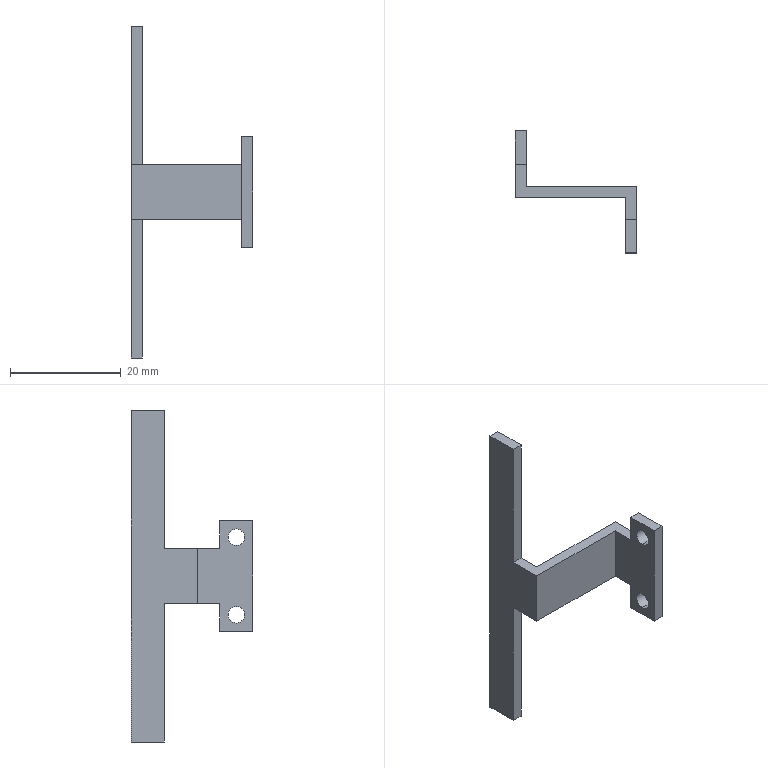Part | SolidWorks | features ICE 2, Extrusion 1 | 1 solid | 22 faces | box 22 x 22 x 60 mm | volume 1532 mm3 | plane 18 | cylinder 4 | commonest cylinder face diameters 3 x4
STEP:
#1=CARTESIAN_POINT('',(3.784,-3.326,8.5));
#2=VERTEX_POINT('',#1);
#3=CARTESIAN_POINT('',(3.784,-3.326,5.5));
#4=VERTEX_POINT('',#3);
#5=CARTESIAN_POINT('',(3.784,-3.326,7.));
#6=DIRECTION('',(1.,0.,0.));
#7=DIRECTION('',(0.,0.,-1.));
#8=AXIS2_PLACEMENT_3D('',#5,#6,#7);
#9=CIRCLE('',#8,1.5);
#10=EDGE_CURVE('',#2,#4,#9,.T.);
#11=ORIENTED_EDGE('',*,*,#10,.F.);
#12=CARTESIAN_POINT('',(5.784,-3.326,8.5));
#13=VERTEX_POINT('',#12);
#14=CARTESIAN_POINT('',(3.784,-3.326,8.5));
#15=DIRECTION('',(1.,0.,0.));
#16=VECTOR('',#15,1000.);
#17=LINE('',#14,#16);
#18=EDGE_CURVE('',#2,#13,#17,.T.);
#19=ORIENTED_EDGE('',*,*,#18,.T.);
#20=CARTESIAN_POINT('',(5.784,-3.326,5.5));
#21=VERTEX_POINT('',#20);
#22=CARTESIAN_POINT('',(5.784,-3.326,7.));
#23=DIRECTION('',(1.,0.,0.));
#24=DIRECTION('',(0.,0.,-1.));
#25=AXIS2_PLACEMENT_3D('',#22,#23,#24);
#26=CIRCLE('',#25,1.5);
#27=EDGE_CURVE('',#13,#21,#26,.T.);
#28=ORIENTED_EDGE('',*,*,#27,.T.);
#29=CARTESIAN_POINT('',(3.784,-3.326,5.5));
#30=DIRECTION('',(1.,0.,0.));
#31=VECTOR('',#30,1000.);
#32=LINE('',#29,#31);
#33=EDGE_CURVE('',#4,#21,#32,.T.);
#34=ORIENTED_EDGE('',*,*,#33,.F.);
#35=EDGE_LOOP('',(#11,#19,#28,#34));
#36=FACE_OUTER_BOUND('',#35,.T.);
#37=CARTESIAN_POINT('',(3.784,-3.326,7.));
#38=DIRECTION('',(1.,0.,0.));
#39=DIRECTION('',(0.,0.,-1.));
#40=AXIS2_PLACEMENT_3D('',#37,#38,#39);
#41=CYLINDRICAL_SURFACE('',#40,1.5);
#42=ADVANCED_FACE('',(#36),#41,.F.);
#43=CARTESIAN_POINT('',(3.784,-3.326,-5.5));
#44=VERTEX_POINT('',#43);
#45=CARTESIAN_POINT('',(3.784,-3.326,-8.5));
#46=VERTEX_POINT('',#45);
#47=CARTESIAN_POINT('',(3.784,-3.326,-7.));
#48=DIRECTION('',(1.,0.,0.));
#49=DIRECTION('',(0.,0.,-1.));
#50=AXIS2_PLACEMENT_3D('',#47,#48,#49);
#51=CIRCLE('',#50,1.5);
#52=EDGE_CURVE('',#44,#46,#51,.T.);
#53=ORIENTED_EDGE('',*,*,#52,.F.);
#54=CARTESIAN_POINT('',(5.784,-3.326,-5.5));
#55=VERTEX_POINT('',#54);
#56=CARTESIAN_POINT('',(3.784,-3.326,-5.5));
#57=DIRECTION('',(1.,0.,0.));
#58=VECTOR('',#57,1000.);
#59=LINE('',#56,#58);
#60=EDGE_CURVE('',#44,#55,#59,.T.);
#61=ORIENTED_EDGE('',*,*,#60,.T.);
#62=CARTESIAN_POINT('',(5.784,-3.326,-8.5));
#63=VERTEX_POINT('',#62);
#64=CARTESIAN_POINT('',(5.784,-3.326,-7.));
#65=DIRECTION('',(1.,0.,0.));
#66=DIRECTION('',(0.,0.,-1.));
#67=AXIS2_PLACEMENT_3D('',#64,#65,#66);
#68=CIRCLE('',#67,1.5);
#69=EDGE_CURVE('',#55,#63,#68,.T.);
#70=ORIENTED_EDGE('',*,*,#69,.T.);
#71=CARTESIAN_POINT('',(3.784,-3.326,-8.5));
#72=DIRECTION('',(1.,0.,0.));
#73=VECTOR('',#72,1000.);
#74=LINE('',#71,#73);
#75=EDGE_CURVE('',#46,#63,#74,.T.);
#76=ORIENTED_EDGE('',*,*,#75,.F.);
#77=EDGE_LOOP('',(#53,#61,#70,#76));
#78=FACE_OUTER_BOUND('',#77,.T.);
#79=CARTESIAN_POINT('',(3.784,-3.326,-7.));
#80=DIRECTION('',(1.,0.,0.));
#81=DIRECTION('',(0.,0.,-1.));
#82=AXIS2_PLACEMENT_3D('',#79,#80,#81);
#83=CYLINDRICAL_SURFACE('',#82,1.5);
#84=ADVANCED_FACE('',(#78),#83,.F.);
#85=CARTESIAN_POINT('',(5.784,-0.3262,5.));
#86=VERTEX_POINT('',#85);
#87=CARTESIAN_POINT('',(5.784,5.674,5.));
#88=VERTEX_POINT('',#87);
#89=CARTESIAN_POINT('',(5.784,5.674,5.));
#90=DIRECTION('',(0.,1.,0.));
#91=VECTOR('',#90,1000.);
#92=LINE('',#89,#91);
#93=EDGE_CURVE('',#86,#88,#92,.T.);
#94=ORIENTED_EDGE('',*,*,#93,.F.);
#95=CARTESIAN_POINT('',(5.784,-0.3262,10.));
#96=VERTEX_POINT('',#95);
#97=CARTESIAN_POINT('',(5.784,-0.3262,-10.));
#98=DIRECTION('',(0.,0.,1.));
#99=VECTOR('',#98,1000.);
#100=LINE('',#97,#99);
#101=EDGE_CURVE('',#86,#96,#100,.T.);
#102=ORIENTED_EDGE('',*,*,#101,.T.);
#103=CARTESIAN_POINT('',(5.784,-6.326,10.));
#104=VERTEX_POINT('',#103);
#105=CARTESIAN_POINT('',(5.784,-0.3262,10.));
#106=DIRECTION('',(0.,-1.,0.));
#107=VECTOR('',#106,1000.);
#108=LINE('',#105,#107);
#109=EDGE_CURVE('',#96,#104,#108,.T.);
#110=ORIENTED_EDGE('',*,*,#109,.T.);
#111=CARTESIAN_POINT('',(5.784,-6.326,-10.));
#112=VERTEX_POINT('',#111);
#113=CARTESIAN_POINT('',(5.784,-6.326,5.));
#114=DIRECTION('',(0.,0.,-1.));
#115=VECTOR('',#114,1000.);
#116=LINE('',#113,#115);
#117=EDGE_CURVE('',#104,#112,#116,.T.);
#118=ORIENTED_EDGE('',*,*,#117,.T.);
#119=CARTESIAN_POINT('',(5.784,-0.3262,-10.));
#120=VERTEX_POINT('',#119);
#121=CARTESIAN_POINT('',(5.784,-6.326,-10.));
#122=DIRECTION('',(0.,1.,0.));
#123=VECTOR('',#122,1000.);
#124=LINE('',#121,#123);
#125=EDGE_CURVE('',#112,#120,#124,.T.);
#126=ORIENTED_EDGE('',*,*,#125,.T.);
#127=CARTESIAN_POINT('',(5.784,-0.3262,-5.));
#128=VERTEX_POINT('',#127);
#129=CARTESIAN_POINT('',(5.784,-0.3262,-10.));
#130=DIRECTION('',(0.,0.,1.));
#131=VECTOR('',#130,1000.);
#132=LINE('',#129,#131);
#133=EDGE_CURVE('',#120,#128,#132,.T.);
#134=ORIENTED_EDGE('',*,*,#133,.T.);
#135=CARTESIAN_POINT('',(5.784,5.674,-5.));
#136=VERTEX_POINT('',#135);
#137=CARTESIAN_POINT('',(5.784,5.674,-5.));
#138=DIRECTION('',(0.,1.,0.));
#139=VECTOR('',#138,1000.);
#140=LINE('',#137,#139);
#141=EDGE_CURVE('',#128,#136,#140,.T.);
#142=ORIENTED_EDGE('',*,*,#141,.T.);
#143=CARTESIAN_POINT('',(5.784,5.674,5.));
#144=DIRECTION('',(0.,0.,-1.));
#145=VECTOR('',#144,1000.);
#146=LINE('',#143,#145);
#147=EDGE_CURVE('',#88,#136,#146,.T.);
#148=ORIENTED_EDGE('',*,*,#147,.F.);
#149=EDGE_LOOP('',(#94,#102,#110,#118,#126,#134,#142,#148));
#150=FACE_OUTER_BOUND('',#149,.T.);
#151=CARTESIAN_POINT('',(5.784,-3.326,-7.));
#152=DIRECTION('',(1.,0.,0.));
#153=DIRECTION('',(0.,0.,-1.));
#154=AXIS2_PLACEMENT_3D('',#151,#152,#153);
#155=CIRCLE('',#154,1.5);
#156=EDGE_CURVE('',#63,#55,#155,.T.);
#157=ORIENTED_EDGE('',*,*,#156,.F.);
#158=ORIENTED_EDGE('',*,*,#69,.F.);
#159=EDGE_LOOP('',(#157,#158));
#160=FACE_BOUND('',#159,.T.);
#161=CARTESIAN_POINT('',(5.784,-3.326,7.));
#162=DIRECTION('',(1.,0.,0.));
#163=DIRECTION('',(0.,0.,-1.));
#164=AXIS2_PLACEMENT_3D('',#161,#162,#163);
#165=CIRCLE('',#164,1.5);
#166=EDGE_CURVE('',#21,#13,#165,.T.);
#167=ORIENTED_EDGE('',*,*,#166,.F.);
#168=ORIENTED_EDGE('',*,*,#27,.F.);
#169=EDGE_LOOP('',(#167,#168));
#170=FACE_BOUND('',#169,.T.);
#171=CARTESIAN_POINT('',(5.784,5.674,5.));
#172=DIRECTION('',(-1.,0.,0.));
#173=DIRECTION('',(0.,0.,1.));
#174=AXIS2_PLACEMENT_3D('',#171,#172,#173);
#175=PLANE('',#174);
#176=ADVANCED_FACE('',(#150,#160,#170),#175,.F.);
#177=CARTESIAN_POINT('',(-14.216,5.674,-5.));
#178=VERTEX_POINT('',#177);
#179=CARTESIAN_POINT('',(-14.216,5.674,-5.));
#180=DIRECTION('',(-1.,0.,0.));
#181=VECTOR('',#180,1000.);
#182=LINE('',#179,#181);
#183=EDGE_CURVE('',#136,#178,#182,.T.);
#184=ORIENTED_EDGE('',*,*,#183,.T.);
#185=CARTESIAN_POINT('',(-14.216,5.674,5.));
#186=VERTEX_POINT('',#185);
#187=CARTESIAN_POINT('',(-14.216,5.674,5.));
#188=DIRECTION('',(0.,0.,-1.));
#189=VECTOR('',#188,1000.);
#190=LINE('',#187,#189);
#191=EDGE_CURVE('',#186,#178,#190,.T.);
#192=ORIENTED_EDGE('',*,*,#191,.F.);
#193=CARTESIAN_POINT('',(-14.216,5.674,5.));
#194=DIRECTION('',(-1.,0.,0.));
#195=VECTOR('',#194,1000.);
#196=LINE('',#193,#195);
#197=EDGE_CURVE('',#88,#186,#196,.T.);
#198=ORIENTED_EDGE('',*,*,#197,.F.);
#199=ORIENTED_EDGE('',*,*,#147,.T.);
#200=EDGE_LOOP('',(#184,#192,#198,#199));
#201=FACE_OUTER_BOUND('',#200,.T.);
#202=CARTESIAN_POINT('',(-14.216,5.674,5.));
#203=DIRECTION('',(0.,-1.,0.));
#204=DIRECTION('',(0.,0.,-1.));
#205=AXIS2_PLACEMENT_3D('',#202,#203,#204);
#206=PLANE('',#205);
#207=ADVANCED_FACE('',(#201),#206,.F.);
#208=CARTESIAN_POINT('',(-14.216,9.674,-5.));
#209=VERTEX_POINT('',#208);
#210=CARTESIAN_POINT('',(-14.216,5.674,-5.));
#211=DIRECTION('',(0.,1.,0.));
#212=VECTOR('',#211,1000.);
#213=LINE('',#210,#212);
#214=EDGE_CURVE('',#178,#209,#213,.T.);
#215=ORIENTED_EDGE('',*,*,#214,.T.);
#216=CARTESIAN_POINT('',(-14.216,9.674,-30.));
#217=VERTEX_POINT('',#216);
#218=CARTESIAN_POINT('',(-14.216,9.674,-30.));
#219=DIRECTION('',(0.,0.,1.));
#220=VECTOR('',#219,1000.);
#221=LINE('',#218,#220);
#222=EDGE_CURVE('',#217,#209,#221,.T.);
#223=ORIENTED_EDGE('',*,*,#222,.F.);
#224=CARTESIAN_POINT('',(-14.216,15.674,-30.));
#225=VERTEX_POINT('',#224);
#226=CARTESIAN_POINT('',(-14.216,15.674,-30.));
#227=DIRECTION('',(0.,-1.,0.));
#228=VECTOR('',#227,1000.);
#229=LINE('',#226,#228);
#230=EDGE_CURVE('',#225,#217,#229,.T.);
#231=ORIENTED_EDGE('',*,*,#230,.F.);
#232=CARTESIAN_POINT('',(-14.216,15.674,30.));
#233=VERTEX_POINT('',#232);
#234=CARTESIAN_POINT('',(-14.216,15.674,5.));
#235=DIRECTION('',(0.,0.,-1.));
#236=VECTOR('',#235,1000.);
#237=LINE('',#234,#236);
#238=EDGE_CURVE('',#233,#225,#237,.T.);
#239=ORIENTED_EDGE('',*,*,#238,.F.);
#240=CARTESIAN_POINT('',(-14.216,9.674,30.));
#241=VERTEX_POINT('',#240);
#242=CARTESIAN_POINT('',(-14.216,15.674,30.));
#243=DIRECTION('',(0.,1.,0.));
#244=VECTOR('',#243,1000.);
#245=LINE('',#242,#244);
#246=EDGE_CURVE('',#241,#233,#245,.T.);
#247=ORIENTED_EDGE('',*,*,#246,.F.);
#248=CARTESIAN_POINT('',(-14.216,9.674,5.));
#249=VERTEX_POINT('',#248);
#250=CARTESIAN_POINT('',(-14.216,9.674,-30.));
#251=DIRECTION('',(0.,0.,1.));
#252=VECTOR('',#251,1000.);
#253=LINE('',#250,#252);
#254=EDGE_CURVE('',#249,#241,#253,.T.);
#255=ORIENTED_EDGE('',*,*,#254,.F.);
#256=CARTESIAN_POINT('',(-14.216,5.674,5.));
#257=DIRECTION('',(0.,1.,0.));
#258=VECTOR('',#257,1000.);
#259=LINE('',#256,#258);
#260=EDGE_CURVE('',#186,#249,#259,.T.);
#261=ORIENTED_EDGE('',*,*,#260,.F.);
#262=ORIENTED_EDGE('',*,*,#191,.T.);
#263=EDGE_LOOP('',(#215,#223,#231,#239,#247,#255,#261,#262));
#264=FACE_OUTER_BOUND('',#263,.T.);
#265=CARTESIAN_POINT('',(-14.216,5.674,5.));
#266=DIRECTION('',(-1.,0.,0.));
#267=DIRECTION('',(0.,0.,1.));
#268=AXIS2_PLACEMENT_3D('',#265,#266,#267);
#269=PLANE('',#268);
#270=ADVANCED_FACE('',(#264),#269,.F.);
#271=ORIENTED_EDGE('',*,*,#238,.T.);
#272=CARTESIAN_POINT('',(-16.216,15.674,-30.));
#273=VERTEX_POINT('',#272);
#274=CARTESIAN_POINT('',(-14.216,15.674,-30.));
#275=DIRECTION('',(-1.,0.,0.));
#276=VECTOR('',#275,1000.);
#277=LINE('',#274,#276);
#278=EDGE_CURVE('',#225,#273,#277,.T.);
#279=ORIENTED_EDGE('',*,*,#278,.T.);
#280=CARTESIAN_POINT('',(-16.216,15.674,30.));
#281=VERTEX_POINT('',#280);
#282=CARTESIAN_POINT('',(-16.216,15.674,5.));
#283=DIRECTION('',(0.,0.,-1.));
#284=VECTOR('',#283,1000.);
#285=LINE('',#282,#284);
#286=EDGE_CURVE('',#281,#273,#285,.T.);
#287=ORIENTED_EDGE('',*,*,#286,.F.);
#288=CARTESIAN_POINT('',(-14.216,15.674,30.));
#289=DIRECTION('',(-1.,0.,0.));
#290=VECTOR('',#289,1000.);
#291=LINE('',#288,#290);
#292=EDGE_CURVE('',#233,#281,#291,.T.);
#293=ORIENTED_EDGE('',*,*,#292,.F.);
#294=EDGE_LOOP('',(#271,#279,#287,#293));
#295=FACE_OUTER_BOUND('',#294,.T.);
#296=CARTESIAN_POINT('',(-16.216,15.674,5.));
#297=DIRECTION('',(0.,-1.,0.));
#298=DIRECTION('',(0.,0.,-1.));
#299=AXIS2_PLACEMENT_3D('',#296,#297,#298);
#300=PLANE('',#299);
#301=ADVANCED_FACE('',(#295),#300,.F.);
#302=CARTESIAN_POINT('',(-16.216,9.674,5.));
#303=VERTEX_POINT('',#302);
#304=CARTESIAN_POINT('',(-16.216,3.674,5.));
#305=VERTEX_POINT('',#304);
#306=CARTESIAN_POINT('',(-16.216,3.674,5.));
#307=DIRECTION('',(0.,-1.,0.));
#308=VECTOR('',#307,1000.);
#309=LINE('',#306,#308);
#310=EDGE_CURVE('',#303,#305,#309,.T.);
#311=ORIENTED_EDGE('',*,*,#310,.F.);
#312=CARTESIAN_POINT('',(-16.216,9.674,30.));
#313=VERTEX_POINT('',#312);
#314=CARTESIAN_POINT('',(-16.216,9.674,-30.));
#315=DIRECTION('',(0.,0.,1.));
#316=VECTOR('',#315,1000.);
#317=LINE('',#314,#316);
#318=EDGE_CURVE('',#303,#313,#317,.T.);
#319=ORIENTED_EDGE('',*,*,#318,.T.);
#320=CARTESIAN_POINT('',(-16.216,15.674,30.));
#321=DIRECTION('',(0.,1.,0.));
#322=VECTOR('',#321,1000.);
#323=LINE('',#320,#322);
#324=EDGE_CURVE('',#313,#281,#323,.T.);
#325=ORIENTED_EDGE('',*,*,#324,.T.);
#326=ORIENTED_EDGE('',*,*,#286,.T.);
#327=CARTESIAN_POINT('',(-16.216,9.674,-30.));
#328=VERTEX_POINT('',#327);
#329=CARTESIAN_POINT('',(-16.216,15.674,-30.));
#330=DIRECTION('',(0.,-1.,0.));
#331=VECTOR('',#330,1000.);
#332=LINE('',#329,#331);
#333=EDGE_CURVE('',#273,#328,#332,.T.);
#334=ORIENTED_EDGE('',*,*,#333,.T.);
#335=CARTESIAN_POINT('',(-16.216,9.674,-5.));
#336=VERTEX_POINT('',#335);
#337=CARTESIAN_POINT('',(-16.216,9.674,-30.));
#338=DIRECTION('',(0.,0.,1.));
#339=VECTOR('',#338,1000.);
#340=LINE('',#337,#339);
#341=EDGE_CURVE('',#328,#336,#340,.T.);
#342=ORIENTED_EDGE('',*,*,#341,.T.);
#343=CARTESIAN_POINT('',(-16.216,3.674,-5.));
#344=VERTEX_POINT('',#343);
#345=CARTESIAN_POINT('',(-16.216,3.674,-5.));
#346=DIRECTION('',(0.,-1.,0.));
#347=VECTOR('',#346,1000.);
#348=LINE('',#345,#347);
#349=EDGE_CURVE('',#336,#344,#348,.T.);
#350=ORIENTED_EDGE('',*,*,#349,.T.);
#351=CARTESIAN_POINT('',(-16.216,3.674,5.));
#352=DIRECTION('',(0.,0.,-1.));
#353=VECTOR('',#352,1000.);
#354=LINE('',#351,#353);
#355=EDGE_CURVE('',#305,#344,#354,.T.);
#356=ORIENTED_EDGE('',*,*,#355,.F.);
#357=EDGE_LOOP('',(#311,#319,#325,#326,#334,#342,#350,#356));
#358=FACE_OUTER_BOUND('',#357,.T.);
#359=CARTESIAN_POINT('',(-16.216,3.674,5.));
#360=DIRECTION('',(1.,0.,0.));
#361=DIRECTION('',(0.,0.,-1.));
#362=AXIS2_PLACEMENT_3D('',#359,#360,#361);
#363=PLANE('',#362);
#364=ADVANCED_FACE('',(#358),#363,.F.);
#365=CARTESIAN_POINT('',(3.784,3.674,-5.));
#366=VERTEX_POINT('',#365);
#367=CARTESIAN_POINT('',(-16.216,3.674,-5.));
#368=DIRECTION('',(1.,0.,0.));
#369=VECTOR('',#368,1000.);
#370=LINE('',#367,#369);
#371=EDGE_CURVE('',#344,#366,#370,.T.);
#372=ORIENTED_EDGE('',*,*,#371,.T.);
#373=CARTESIAN_POINT('',(3.784,3.674,5.));
#374=VERTEX_POINT('',#373);
#375=CARTESIAN_POINT('',(3.784,3.674,5.));
#376=DIRECTION('',(0.,0.,-1.));
#377=VECTOR('',#376,1000.);
#378=LINE('',#375,#377);
#379=EDGE_CURVE('',#374,#366,#378,.T.);
#380=ORIENTED_EDGE('',*,*,#379,.F.);
#381=CARTESIAN_POINT('',(-16.216,3.674,5.));
#382=DIRECTION('',(1.,0.,0.));
#383=VECTOR('',#382,1000.);
#384=LINE('',#381,#383);
#385=EDGE_CURVE('',#305,#374,#384,.T.);
#386=ORIENTED_EDGE('',*,*,#385,.F.);
#387=ORIENTED_EDGE('',*,*,#355,.T.);
#388=EDGE_LOOP('',(#372,#380,#386,#387));
#389=FACE_OUTER_BOUND('',#388,.T.);
#390=CARTESIAN_POINT('',(-16.216,3.674,5.));
#391=DIRECTION('',(0.,1.,0.));
#392=DIRECTION('',(-1.,0.,0.));
#393=AXIS2_PLACEMENT_3D('',#390,#391,#392);
#394=PLANE('',#393);
#395=ADVANCED_FACE('',(#389),#394,.F.);
#396=CARTESIAN_POINT('',(3.784,-0.3262,-5.));
#397=VERTEX_POINT('',#396);
#398=CARTESIAN_POINT('',(3.784,-6.326,-5.));
#399=DIRECTION('',(0.,-1.,0.));
#400=VECTOR('',#399,1000.);
#401=LINE('',#398,#400);
#402=EDGE_CURVE('',#366,#397,#401,.T.);
#403=ORIENTED_EDGE('',*,*,#402,.T.);
#404=CARTESIAN_POINT('',(3.784,-0.3262,-10.));
#405=VERTEX_POINT('',#404);
#406=CARTESIAN_POINT('',(3.784,-0.3262,-10.));
#407=DIRECTION('',(0.,0.,1.));
#408=VECTOR('',#407,1000.);
#409=LINE('',#406,#408);
#410=EDGE_CURVE('',#405,#397,#409,.T.);
#411=ORIENTED_EDGE('',*,*,#410,.F.);
#412=CARTESIAN_POINT('',(3.784,-6.326,-10.));
#413=VERTEX_POINT('',#412);
#414=CARTESIAN_POINT('',(3.784,-6.326,-10.));
#415=DIRECTION('',(0.,1.,0.));
#416=VECTOR('',#415,1000.);
#417=LINE('',#414,#416);
#418=EDGE_CURVE('',#413,#405,#417,.T.);
#419=ORIENTED_EDGE('',*,*,#418,.F.);
#420=CARTESIAN_POINT('',(3.784,-6.326,10.));
#421=VERTEX_POINT('',#420);
#422=CARTESIAN_POINT('',(3.784,-6.326,5.));
#423=DIRECTION('',(0.,0.,-1.));
#424=VECTOR('',#423,1000.);
#425=LINE('',#422,#424);
#426=EDGE_CURVE('',#421,#413,#425,.T.);
#427=ORIENTED_EDGE('',*,*,#426,.F.);
#428=CARTESIAN_POINT('',(3.784,-0.3262,10.));
#429=VERTEX_POINT('',#428);
#430=CARTESIAN_POINT('',(3.784,-0.3262,10.));
#431=DIRECTION('',(0.,-1.,0.));
#432=VECTOR('',#431,1000.);
#433=LINE('',#430,#432);
#434=EDGE_CURVE('',#429,#421,#433,.T.);
#435=ORIENTED_EDGE('',*,*,#434,.F.);
#436=CARTESIAN_POINT('',(3.784,-0.3262,5.));
#437=VERTEX_POINT('',#436);
#438=CARTESIAN_POINT('',(3.784,-0.3262,-10.));
#439=DIRECTION('',(0.,0.,1.));
#440=VECTOR('',#439,1000.);
#441=LINE('',#438,#440);
#442=EDGE_CURVE('',#437,#429,#441,.T.);
#443=ORIENTED_EDGE('',*,*,#442,.F.);
#444=CARTESIAN_POINT('',(3.784,-6.326,5.));
#445=DIRECTION('',(0.,-1.,0.));
#446=VECTOR('',#445,1000.);
#447=LINE('',#444,#446);
#448=EDGE_CURVE('',#374,#437,#447,.T.);
#449=ORIENTED_EDGE('',*,*,#448,.F.);
#450=ORIENTED_EDGE('',*,*,#379,.T.);
#451=EDGE_LOOP('',(#403,#411,#419,#427,#435,#443,#449,#450));
#452=FACE_OUTER_BOUND('',#451,.T.);
#453=CARTESIAN_POINT('',(3.784,-3.326,-7.));
#454=DIRECTION('',(1.,0.,0.));
#455=DIRECTION('',(0.,0.,-1.));
#456=AXIS2_PLACEMENT_3D('',#453,#454,#455);
#457=CIRCLE('',#456,1.5);
#458=EDGE_CURVE('',#46,#44,#457,.T.);
#459=ORIENTED_EDGE('',*,*,#458,.T.);
#460=ORIENTED_EDGE('',*,*,#52,.T.);
#461=EDGE_LOOP('',(#459,#460));
#462=FACE_BOUND('',#461,.T.);
#463=CARTESIAN_POINT('',(3.784,-3.326,7.));
#464=DIRECTION('',(1.,0.,0.));
#465=DIRECTION('',(0.,0.,-1.));
#466=AXIS2_PLACEMENT_3D('',#463,#464,#465);
#467=CIRCLE('',#466,1.5);
#468=EDGE_CURVE('',#4,#2,#467,.T.);
#469=ORIENTED_EDGE('',*,*,#468,.T.);
#470=ORIENTED_EDGE('',*,*,#10,.T.);
#471=EDGE_LOOP('',(#469,#470));
#472=FACE_BOUND('',#471,.T.);
#473=CARTESIAN_POINT('',(3.784,-6.326,5.));
#474=DIRECTION('',(1.,0.,0.));
#475=DIRECTION('',(0.,0.,-1.));
#476=AXIS2_PLACEMENT_3D('',#473,#474,#475);
#477=PLANE('',#476);
#478=ADVANCED_FACE('',(#452,#462,#472),#477,.F.);
#479=ORIENTED_EDGE('',*,*,#426,.T.);
#480=CARTESIAN_POINT('',(3.784,-6.326,-10.));
#481=DIRECTION('',(1.,0.,0.));
#482=VECTOR('',#481,1000.);
#483=LINE('',#480,#482);
#484=EDGE_CURVE('',#413,#112,#483,.T.);
#485=ORIENTED_EDGE('',*,*,#484,.T.);
#486=ORIENTED_EDGE('',*,*,#117,.F.);
#487=CARTESIAN_POINT('',(3.784,-6.326,10.));
#488=DIRECTION('',(1.,0.,0.));
#489=VECTOR('',#488,1000.);
#490=LINE('',#487,#489);
#491=EDGE_CURVE('',#421,#104,#490,.T.);
#492=ORIENTED_EDGE('',*,*,#491,.F.);
#493=EDGE_LOOP('',(#479,#485,#486,#492));
#494=FACE_OUTER_BOUND('',#493,.T.);
#495=CARTESIAN_POINT('',(5.784,-6.326,5.));
#496=DIRECTION('',(0.,1.,0.));
#497=DIRECTION('',(0.,0.,1.));
#498=AXIS2_PLACEMENT_3D('',#495,#496,#497);
#499=PLANE('',#498);
#500=ADVANCED_FACE('',(#494),#499,.F.);
#501=ORIENTED_EDGE('',*,*,#260,.T.);
#502=CARTESIAN_POINT('',(0.,9.674,5.));
#503=DIRECTION('',(-1.,0.,0.));
#504=VECTOR('',#503,1000.);
#505=LINE('',#502,#504);
#506=EDGE_CURVE('',#249,#303,#505,.T.);
#507=ORIENTED_EDGE('',*,*,#506,.T.);
#508=ORIENTED_EDGE('',*,*,#310,.T.);
#509=ORIENTED_EDGE('',*,*,#385,.T.);
#510=ORIENTED_EDGE('',*,*,#448,.T.);
#511=CARTESIAN_POINT('',(0.,-0.3262,5.));
#512=DIRECTION('',(1.,0.,0.));
#513=VECTOR('',#512,1000.);
#514=LINE('',#511,#513);
#515=EDGE_CURVE('',#437,#86,#514,.T.);
#516=ORIENTED_EDGE('',*,*,#515,.T.);
#517=ORIENTED_EDGE('',*,*,#93,.T.);
#518=ORIENTED_EDGE('',*,*,#197,.T.);
#519=EDGE_LOOP('',(#501,#507,#508,#509,#510,#516,#517,#518));
#520=FACE_OUTER_BOUND('',#519,.T.);
#521=CARTESIAN_POINT('',(0.,0.,5.));
#522=DIRECTION('',(0.,0.,-1.));
#523=DIRECTION('',(-1.,0.,0.));
#524=AXIS2_PLACEMENT_3D('',#521,#522,#523);
#525=PLANE('',#524);
#526=ADVANCED_FACE('',(#520),#525,.F.);
#527=CARTESIAN_POINT('',(0.,9.674,-5.));
#528=DIRECTION('',(-1.,0.,0.));
#529=VECTOR('',#528,1000.);
#530=LINE('',#527,#529);
#531=EDGE_CURVE('',#209,#336,#530,.T.);
#532=ORIENTED_EDGE('',*,*,#531,.F.);
#533=ORIENTED_EDGE('',*,*,#214,.F.);
#534=ORIENTED_EDGE('',*,*,#183,.F.);
#535=ORIENTED_EDGE('',*,*,#141,.F.);
#536=CARTESIAN_POINT('',(0.,-0.3262,-5.));
#537=DIRECTION('',(1.,0.,0.));
#538=VECTOR('',#537,1000.);
#539=LINE('',#536,#538);
#540=EDGE_CURVE('',#397,#128,#539,.T.);
#541=ORIENTED_EDGE('',*,*,#540,.F.);
#542=ORIENTED_EDGE('',*,*,#402,.F.);
#543=ORIENTED_EDGE('',*,*,#371,.F.);
#544=ORIENTED_EDGE('',*,*,#349,.F.);
#545=EDGE_LOOP('',(#532,#533,#534,#535,#541,#542,#543,#544));
#546=FACE_OUTER_BOUND('',#545,.T.);
#547=CARTESIAN_POINT('',(0.,0.,-5.));
#548=DIRECTION('',(0.,0.,-1.));
#549=DIRECTION('',(-1.,0.,0.));
#550=AXIS2_PLACEMENT_3D('',#547,#548,#549);
#551=PLANE('',#550);
#552=ADVANCED_FACE('',(#546),#551,.T.);
#553=ORIENTED_EDGE('',*,*,#125,.F.);
#554=ORIENTED_EDGE('',*,*,#484,.F.);
#555=ORIENTED_EDGE('',*,*,#418,.T.);
#556=CARTESIAN_POINT('',(3.784,-0.3262,-10.));
#557=DIRECTION('',(1.,0.,0.));
#558=VECTOR('',#557,1000.);
#559=LINE('',#556,#558);
#560=EDGE_CURVE('',#405,#120,#559,.T.);
#561=ORIENTED_EDGE('',*,*,#560,.T.);
#562=EDGE_LOOP('',(#553,#554,#555,#561));
#563=FACE_OUTER_BOUND('',#562,.T.);
#564=CARTESIAN_POINT('',(3.784,-6.326,-10.));
#565=DIRECTION('',(0.,0.,-1.));
#566=DIRECTION('',(0.,1.,0.));
#567=AXIS2_PLACEMENT_3D('',#564,#565,#566);
#568=PLANE('',#567);
#569=ADVANCED_FACE('',(#563),#568,.T.);
#570=ORIENTED_EDGE('',*,*,#60,.F.);
#571=ORIENTED_EDGE('',*,*,#458,.F.);
#572=ORIENTED_EDGE('',*,*,#75,.T.);
#573=ORIENTED_EDGE('',*,*,#156,.T.);
#574=EDGE_LOOP('',(#570,#571,#572,#573));
#575=FACE_OUTER_BOUND('',#574,.T.);
#576=CARTESIAN_POINT('',(3.784,-3.326,-7.));
#577=DIRECTION('',(1.,0.,0.));
#578=DIRECTION('',(0.,0.,-1.));
#579=AXIS2_PLACEMENT_3D('',#576,#577,#578);
#580=CYLINDRICAL_SURFACE('',#579,1.5);
#581=ADVANCED_FACE('',(#575),#580,.F.);
#582=ORIENTED_EDGE('',*,*,#410,.T.);
#583=ORIENTED_EDGE('',*,*,#540,.T.);
#584=ORIENTED_EDGE('',*,*,#133,.F.);
#585=ORIENTED_EDGE('',*,*,#560,.F.);
#586=EDGE_LOOP('',(#582,#583,#584,#585));
#587=FACE_OUTER_BOUND('',#586,.T.);
#588=CARTESIAN_POINT('',(3.784,-0.3262,-10.));
#589=DIRECTION('',(0.,1.,0.));
#590=DIRECTION('',(0.,0.,1.));
#591=AXIS2_PLACEMENT_3D('',#588,#589,#590);
#592=PLANE('',#591);
#593=ADVANCED_FACE('',(#587),#592,.T.);
#594=ORIENTED_EDGE('',*,*,#515,.F.);
#595=ORIENTED_EDGE('',*,*,#442,.T.);
#596=CARTESIAN_POINT('',(3.784,-0.3262,10.));
#597=DIRECTION('',(1.,0.,0.));
#598=VECTOR('',#597,1000.);
#599=LINE('',#596,#598);
#600=EDGE_CURVE('',#429,#96,#599,.T.);
#601=ORIENTED_EDGE('',*,*,#600,.T.);
#602=ORIENTED_EDGE('',*,*,#101,.F.);
#603=EDGE_LOOP('',(#594,#595,#601,#602));
#604=FACE_OUTER_BOUND('',#603,.T.);
#605=CARTESIAN_POINT('',(3.784,-0.3262,-10.));
#606=DIRECTION('',(0.,1.,0.));
#607=DIRECTION('',(0.,0.,1.));
#608=AXIS2_PLACEMENT_3D('',#605,#606,#607);
#609=PLANE('',#608);
#610=ADVANCED_FACE('',(#604),#609,.T.);
#611=ORIENTED_EDGE('',*,*,#109,.F.);
#612=ORIENTED_EDGE('',*,*,#600,.F.);
#613=ORIENTED_EDGE('',*,*,#434,.T.);
#614=ORIENTED_EDGE('',*,*,#491,.T.);
#615=EDGE_LOOP('',(#611,#612,#613,#614));
#616=FACE_OUTER_BOUND('',#615,.T.);
#617=CARTESIAN_POINT('',(3.784,-0.3262,10.));
#618=DIRECTION('',(0.,0.,1.));
#619=DIRECTION('',(0.,-1.,0.));
#620=AXIS2_PLACEMENT_3D('',#617,#618,#619);
#621=PLANE('',#620);
#622=ADVANCED_FACE('',(#616),#621,.T.);
#623=ORIENTED_EDGE('',*,*,#18,.F.);
#624=ORIENTED_EDGE('',*,*,#468,.F.);
#625=ORIENTED_EDGE('',*,*,#33,.T.);
#626=ORIENTED_EDGE('',*,*,#166,.T.);
#627=EDGE_LOOP('',(#623,#624,#625,#626));
#628=FACE_OUTER_BOUND('',#627,.T.);
#629=CARTESIAN_POINT('',(3.784,-3.326,7.));
#630=DIRECTION('',(1.,0.,0.));
#631=DIRECTION('',(0.,0.,-1.));
#632=AXIS2_PLACEMENT_3D('',#629,#630,#631);
#633=CYLINDRICAL_SURFACE('',#632,1.5);
#634=ADVANCED_FACE('',(#628),#633,.F.);
#635=ORIENTED_EDGE('',*,*,#333,.F.);
#636=ORIENTED_EDGE('',*,*,#278,.F.);
#637=ORIENTED_EDGE('',*,*,#230,.T.);
#638=CARTESIAN_POINT('',(-14.216,9.674,-30.));
#639=DIRECTION('',(-1.,0.,0.));
#640=VECTOR('',#639,1000.);
#641=LINE('',#638,#640);
#642=EDGE_CURVE('',#217,#328,#641,.T.);
#643=ORIENTED_EDGE('',*,*,#642,.T.);
#644=EDGE_LOOP('',(#635,#636,#637,#643));
#645=FACE_OUTER_BOUND('',#644,.T.);
#646=CARTESIAN_POINT('',(-14.216,15.674,-30.));
#647=DIRECTION('',(0.,0.,-1.));
#648=DIRECTION('',(-1.,0.,0.));
#649=AXIS2_PLACEMENT_3D('',#646,#647,#648);
#650=PLANE('',#649);
#651=ADVANCED_FACE('',(#645),#650,.T.);
#652=ORIENTED_EDGE('',*,*,#222,.T.);
#653=ORIENTED_EDGE('',*,*,#531,.T.);
#654=ORIENTED_EDGE('',*,*,#341,.F.);
#655=ORIENTED_EDGE('',*,*,#642,.F.);
#656=EDGE_LOOP('',(#652,#653,#654,#655));
#657=FACE_OUTER_BOUND('',#656,.T.);
#658=CARTESIAN_POINT('',(-14.216,9.674,-30.));
#659=DIRECTION('',(0.,-1.,0.));
#660=DIRECTION('',(0.,0.,-1.));
#661=AXIS2_PLACEMENT_3D('',#658,#659,#660);
#662=PLANE('',#661);
#663=ADVANCED_FACE('',(#657),#662,.T.);
#664=ORIENTED_EDGE('',*,*,#506,.F.);
#665=ORIENTED_EDGE('',*,*,#254,.T.);
#666=CARTESIAN_POINT('',(-14.216,9.674,30.));
#667=DIRECTION('',(-1.,0.,0.));
#668=VECTOR('',#667,1000.);
#669=LINE('',#666,#668);
#670=EDGE_CURVE('',#241,#313,#669,.T.);
#671=ORIENTED_EDGE('',*,*,#670,.T.);
#672=ORIENTED_EDGE('',*,*,#318,.F.);
#673=EDGE_LOOP('',(#664,#665,#671,#672));
#674=FACE_OUTER_BOUND('',#673,.T.);
#675=CARTESIAN_POINT('',(-14.216,9.674,-30.));
#676=DIRECTION('',(0.,-1.,0.));
#677=DIRECTION('',(0.,0.,-1.));
#678=AXIS2_PLACEMENT_3D('',#675,#676,#677);
#679=PLANE('',#678);
#680=ADVANCED_FACE('',(#674),#679,.T.);
#681=ORIENTED_EDGE('',*,*,#324,.F.);
#682=ORIENTED_EDGE('',*,*,#670,.F.);
#683=ORIENTED_EDGE('',*,*,#246,.T.);
#684=ORIENTED_EDGE('',*,*,#292,.T.);
#685=EDGE_LOOP('',(#681,#682,#683,#684));
#686=FACE_OUTER_BOUND('',#685,.T.);
#687=CARTESIAN_POINT('',(-14.216,15.674,30.));
#688=DIRECTION('',(0.,0.,1.));
#689=DIRECTION('',(0.,-1.,0.));
#690=AXIS2_PLACEMENT_3D('',#687,#688,#689);
#691=PLANE('',#690);
#692=ADVANCED_FACE('',(#686),#691,.T.);
#693=CLOSED_SHELL('',(#42,#84,#176,#207,#270,#301,#364,#395,#478,#500,#526,#552,#569,#581,#593,#610,#622,#634,#651,#663,#680,#692));
#694=MANIFOLD_SOLID_BREP('',#693);
#695=CARTESIAN_POINT('',(0.,0.,0.));
#696=DIRECTION('',(0.,0.,1.));
#697=DIRECTION('',(1.,0.,0.));
#698=AXIS2_PLACEMENT_3D('',#695,#696,#697);
#699=(LENGTH_UNIT()NAMED_UNIT(*)SI_UNIT(.MILLI.,.METRE.));
#700=UNCERTAINTY_MEASURE_WITH_UNIT(LENGTH_MEASURE(0.00001),#699,'','');
#701=(NAMED_UNIT(*)PLANE_ANGLE_UNIT()SI_UNIT($,.RADIAN.));
#702=(NAMED_UNIT(*)SI_UNIT($,.STERADIAN.)SOLID_ANGLE_UNIT());
#703=(GEOMETRIC_REPRESENTATION_CONTEXT(3)GLOBAL_UNCERTAINTY_ASSIGNED_CONTEXT((#700))GLOBAL_UNIT_ASSIGNED_CONTEXT((#699,#701,#702))REPRESENTATION_CONTEXT('',''));
#704=ADVANCED_BREP_SHAPE_REPRESENTATION('',(#694,#698),#703);